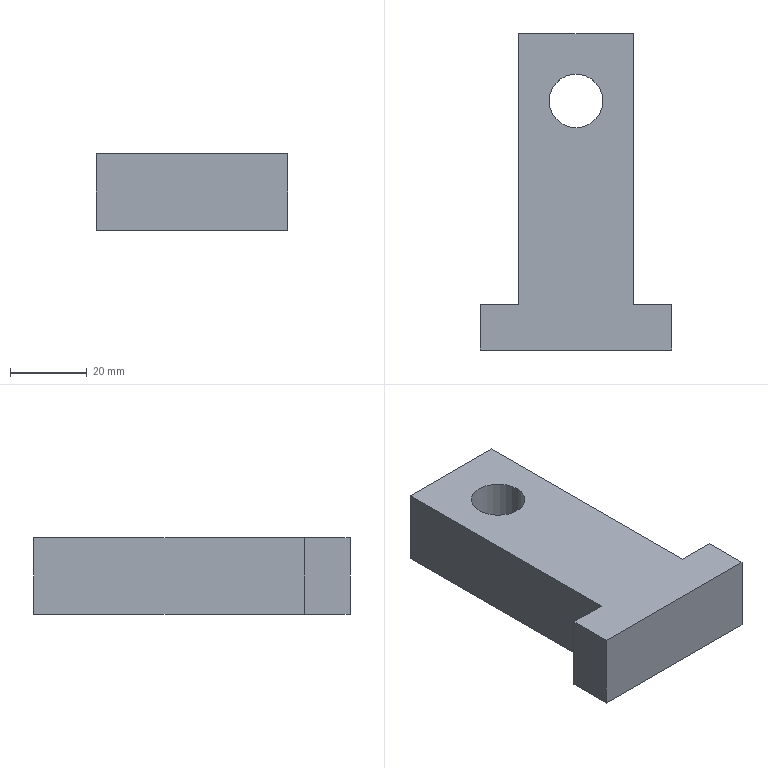Part | SolidWorks | features ICE 2, Extrusion 1 | 1 solid | 12 faces | box 50 x 82.5 x 20 mm | volume 51221 mm3 | plane 10 | cylinder 2 | commonest cylinder face diameters 14 x2
STEP:
#1=CARTESIAN_POINT('',(-7.,23.75,0.));
#2=VERTEX_POINT('',#1);
#3=CARTESIAN_POINT('',(7.,23.75,0.));
#4=VERTEX_POINT('',#3);
#5=CARTESIAN_POINT('',(0.,23.75,0.));
#6=DIRECTION('',(0.,0.,1.));
#7=DIRECTION('',(1.,0.,0.));
#8=AXIS2_PLACEMENT_3D('',#5,#6,#7);
#9=CIRCLE('',#8,7.);
#10=EDGE_CURVE('',#2,#4,#9,.T.);
#11=ORIENTED_EDGE('',*,*,#10,.F.);
#12=CARTESIAN_POINT('',(-7.,23.75,20.));
#13=VERTEX_POINT('',#12);
#14=CARTESIAN_POINT('',(-7.,23.75,0.));
#15=DIRECTION('',(0.,0.,1.));
#16=VECTOR('',#15,1000.);
#17=LINE('',#14,#16);
#18=EDGE_CURVE('',#2,#13,#17,.T.);
#19=ORIENTED_EDGE('',*,*,#18,.T.);
#20=CARTESIAN_POINT('',(7.,23.75,20.));
#21=VERTEX_POINT('',#20);
#22=CARTESIAN_POINT('',(0.,23.75,20.));
#23=DIRECTION('',(0.,0.,1.));
#24=DIRECTION('',(1.,0.,0.));
#25=AXIS2_PLACEMENT_3D('',#22,#23,#24);
#26=CIRCLE('',#25,7.);
#27=EDGE_CURVE('',#13,#21,#26,.T.);
#28=ORIENTED_EDGE('',*,*,#27,.T.);
#29=CARTESIAN_POINT('',(7.,23.75,0.));
#30=DIRECTION('',(0.,0.,1.));
#31=VECTOR('',#30,1000.);
#32=LINE('',#29,#31);
#33=EDGE_CURVE('',#4,#21,#32,.T.);
#34=ORIENTED_EDGE('',*,*,#33,.F.);
#35=EDGE_LOOP('',(#11,#19,#28,#34));
#36=FACE_OUTER_BOUND('',#35,.T.);
#37=CARTESIAN_POINT('',(0.,23.75,0.));
#38=DIRECTION('',(0.,0.,1.));
#39=DIRECTION('',(1.,0.,0.));
#40=AXIS2_PLACEMENT_3D('',#37,#38,#39);
#41=CYLINDRICAL_SURFACE('',#40,7.);
#42=ADVANCED_FACE('',(#36),#41,.F.);
#43=CARTESIAN_POINT('',(25.,-41.25,0.));
#44=VERTEX_POINT('',#43);
#45=CARTESIAN_POINT('',(25.,-29.25,0.));
#46=VERTEX_POINT('',#45);
#47=CARTESIAN_POINT('',(25.,-41.25,0.));
#48=DIRECTION('',(0.,1.,0.));
#49=VECTOR('',#48,1000.);
#50=LINE('',#47,#49);
#51=EDGE_CURVE('',#44,#46,#50,.T.);
#52=ORIENTED_EDGE('',*,*,#51,.T.);
#53=CARTESIAN_POINT('',(25.,-29.25,20.));
#54=VERTEX_POINT('',#53);
#55=CARTESIAN_POINT('',(25.,-29.25,0.));
#56=DIRECTION('',(0.,0.,1.));
#57=VECTOR('',#56,1000.);
#58=LINE('',#55,#57);
#59=EDGE_CURVE('',#46,#54,#58,.T.);
#60=ORIENTED_EDGE('',*,*,#59,.T.);
#61=CARTESIAN_POINT('',(25.,-41.25,20.));
#62=VERTEX_POINT('',#61);
#63=CARTESIAN_POINT('',(25.,-41.25,20.));
#64=DIRECTION('',(0.,1.,0.));
#65=VECTOR('',#64,1000.);
#66=LINE('',#63,#65);
#67=EDGE_CURVE('',#62,#54,#66,.T.);
#68=ORIENTED_EDGE('',*,*,#67,.F.);
#69=CARTESIAN_POINT('',(25.,-41.25,20.));
#70=DIRECTION('',(0.,0.,-1.));
#71=VECTOR('',#70,1000.);
#72=LINE('',#69,#71);
#73=EDGE_CURVE('',#62,#44,#72,.T.);
#74=ORIENTED_EDGE('',*,*,#73,.T.);
#75=EDGE_LOOP('',(#52,#60,#68,#74));
#76=FACE_OUTER_BOUND('',#75,.T.);
#77=CARTESIAN_POINT('',(25.,-41.25,20.));
#78=DIRECTION('',(-1.,0.,0.));
#79=DIRECTION('',(0.,0.,1.));
#80=AXIS2_PLACEMENT_3D('',#77,#78,#79);
#81=PLANE('',#80);
#82=ADVANCED_FACE('',(#76),#81,.F.);
#83=CARTESIAN_POINT('',(15.,41.25,0.));
#84=VERTEX_POINT('',#83);
#85=CARTESIAN_POINT('',(-15.,41.25,0.));
#86=VERTEX_POINT('',#85);
#87=CARTESIAN_POINT('',(-25.,41.25,0.));
#88=DIRECTION('',(-1.,0.,0.));
#89=VECTOR('',#88,1000.);
#90=LINE('',#87,#89);
#91=EDGE_CURVE('',#84,#86,#90,.T.);
#92=ORIENTED_EDGE('',*,*,#91,.T.);
#93=CARTESIAN_POINT('',(-15.,41.25,20.));
#94=VERTEX_POINT('',#93);
#95=CARTESIAN_POINT('',(-15.,41.25,0.));
#96=DIRECTION('',(0.,0.,1.));
#97=VECTOR('',#96,1000.);
#98=LINE('',#95,#97);
#99=EDGE_CURVE('',#86,#94,#98,.T.);
#100=ORIENTED_EDGE('',*,*,#99,.T.);
#101=CARTESIAN_POINT('',(15.,41.25,20.));
#102=VERTEX_POINT('',#101);
#103=CARTESIAN_POINT('',(-25.,41.25,20.));
#104=DIRECTION('',(-1.,0.,0.));
#105=VECTOR('',#104,1000.);
#106=LINE('',#103,#105);
#107=EDGE_CURVE('',#102,#94,#106,.T.);
#108=ORIENTED_EDGE('',*,*,#107,.F.);
#109=CARTESIAN_POINT('',(15.,41.25,0.));
#110=DIRECTION('',(0.,0.,1.));
#111=VECTOR('',#110,1000.);
#112=LINE('',#109,#111);
#113=EDGE_CURVE('',#84,#102,#112,.T.);
#114=ORIENTED_EDGE('',*,*,#113,.F.);
#115=EDGE_LOOP('',(#92,#100,#108,#114));
#116=FACE_OUTER_BOUND('',#115,.T.);
#117=CARTESIAN_POINT('',(-25.,41.25,20.));
#118=DIRECTION('',(0.,-1.,0.));
#119=DIRECTION('',(0.,0.,-1.));
#120=AXIS2_PLACEMENT_3D('',#117,#118,#119);
#121=PLANE('',#120);
#122=ADVANCED_FACE('',(#116),#121,.F.);
#123=CARTESIAN_POINT('',(-25.,-29.25,20.));
#124=VERTEX_POINT('',#123);
#125=CARTESIAN_POINT('',(-25.,-41.25,20.));
#126=VERTEX_POINT('',#125);
#127=CARTESIAN_POINT('',(-25.,-41.25,20.));
#128=DIRECTION('',(0.,-1.,0.));
#129=VECTOR('',#128,1000.);
#130=LINE('',#127,#129);
#131=EDGE_CURVE('',#124,#126,#130,.T.);
#132=ORIENTED_EDGE('',*,*,#131,.F.);
#133=CARTESIAN_POINT('',(-25.,-29.25,0.));
#134=VERTEX_POINT('',#133);
#135=CARTESIAN_POINT('',(-25.,-29.25,0.));
#136=DIRECTION('',(0.,0.,1.));
#137=VECTOR('',#136,1000.);
#138=LINE('',#135,#137);
#139=EDGE_CURVE('',#134,#124,#138,.T.);
#140=ORIENTED_EDGE('',*,*,#139,.F.);
#141=CARTESIAN_POINT('',(-25.,-41.25,0.));
#142=VERTEX_POINT('',#141);
#143=CARTESIAN_POINT('',(-25.,-41.25,0.));
#144=DIRECTION('',(0.,-1.,0.));
#145=VECTOR('',#144,1000.);
#146=LINE('',#143,#145);
#147=EDGE_CURVE('',#134,#142,#146,.T.);
#148=ORIENTED_EDGE('',*,*,#147,.T.);
#149=CARTESIAN_POINT('',(-25.,-41.25,20.));
#150=DIRECTION('',(0.,0.,-1.));
#151=VECTOR('',#150,1000.);
#152=LINE('',#149,#151);
#153=EDGE_CURVE('',#126,#142,#152,.T.);
#154=ORIENTED_EDGE('',*,*,#153,.F.);
#155=EDGE_LOOP('',(#132,#140,#148,#154));
#156=FACE_OUTER_BOUND('',#155,.T.);
#157=CARTESIAN_POINT('',(-25.,-41.25,20.));
#158=DIRECTION('',(1.,0.,0.));
#159=DIRECTION('',(0.,0.,-1.));
#160=AXIS2_PLACEMENT_3D('',#157,#158,#159);
#161=PLANE('',#160);
#162=ADVANCED_FACE('',(#156),#161,.F.);
#163=CARTESIAN_POINT('',(-25.,-41.25,0.));
#164=DIRECTION('',(1.,0.,0.));
#165=VECTOR('',#164,1000.);
#166=LINE('',#163,#165);
#167=EDGE_CURVE('',#142,#44,#166,.T.);
#168=ORIENTED_EDGE('',*,*,#167,.T.);
#169=ORIENTED_EDGE('',*,*,#73,.F.);
#170=CARTESIAN_POINT('',(-25.,-41.25,20.));
#171=DIRECTION('',(1.,0.,0.));
#172=VECTOR('',#171,1000.);
#173=LINE('',#170,#172);
#174=EDGE_CURVE('',#126,#62,#173,.T.);
#175=ORIENTED_EDGE('',*,*,#174,.F.);
#176=ORIENTED_EDGE('',*,*,#153,.T.);
#177=EDGE_LOOP('',(#168,#169,#175,#176));
#178=FACE_OUTER_BOUND('',#177,.T.);
#179=CARTESIAN_POINT('',(-25.,-41.25,20.));
#180=DIRECTION('',(0.,1.,0.));
#181=DIRECTION('',(0.,0.,1.));
#182=AXIS2_PLACEMENT_3D('',#179,#180,#181);
#183=PLANE('',#182);
#184=ADVANCED_FACE('',(#178),#183,.F.);
#185=CARTESIAN_POINT('',(0.,23.75,20.));
#186=DIRECTION('',(0.,0.,1.));
#187=DIRECTION('',(1.,0.,0.));
#188=AXIS2_PLACEMENT_3D('',#185,#186,#187);
#189=CIRCLE('',#188,7.);
#190=EDGE_CURVE('',#21,#13,#189,.T.);
#191=ORIENTED_EDGE('',*,*,#190,.F.);
#192=ORIENTED_EDGE('',*,*,#27,.F.);
#193=EDGE_LOOP('',(#191,#192));
#194=FACE_BOUND('',#193,.T.);
#195=ORIENTED_EDGE('',*,*,#107,.T.);
#196=CARTESIAN_POINT('',(-15.,-29.25,20.));
#197=VERTEX_POINT('',#196);
#198=CARTESIAN_POINT('',(-15.,41.25,20.));
#199=DIRECTION('',(0.,1.,0.));
#200=VECTOR('',#199,1000.);
#201=LINE('',#198,#200);
#202=EDGE_CURVE('',#197,#94,#201,.T.);
#203=ORIENTED_EDGE('',*,*,#202,.F.);
#204=CARTESIAN_POINT('',(-25.,-29.25,20.));
#205=DIRECTION('',(1.,0.,0.));
#206=VECTOR('',#205,1000.);
#207=LINE('',#204,#206);
#208=EDGE_CURVE('',#124,#197,#207,.T.);
#209=ORIENTED_EDGE('',*,*,#208,.F.);
#210=ORIENTED_EDGE('',*,*,#131,.T.);
#211=ORIENTED_EDGE('',*,*,#174,.T.);
#212=ORIENTED_EDGE('',*,*,#67,.T.);
#213=CARTESIAN_POINT('',(15.,-29.25,20.));
#214=VERTEX_POINT('',#213);
#215=CARTESIAN_POINT('',(25.,-29.25,20.));
#216=DIRECTION('',(1.,0.,0.));
#217=VECTOR('',#216,1000.);
#218=LINE('',#215,#217);
#219=EDGE_CURVE('',#214,#54,#218,.T.);
#220=ORIENTED_EDGE('',*,*,#219,.F.);
#221=CARTESIAN_POINT('',(15.,41.25,20.));
#222=DIRECTION('',(0.,-1.,0.));
#223=VECTOR('',#222,1000.);
#224=LINE('',#221,#223);
#225=EDGE_CURVE('',#102,#214,#224,.T.);
#226=ORIENTED_EDGE('',*,*,#225,.F.);
#227=EDGE_LOOP('',(#195,#203,#209,#210,#211,#212,#220,#226));
#228=FACE_OUTER_BOUND('',#227,.T.);
#229=CARTESIAN_POINT('',(0.,0.,20.));
#230=DIRECTION('',(0.,0.,-1.));
#231=DIRECTION('',(-1.,0.,0.));
#232=AXIS2_PLACEMENT_3D('',#229,#230,#231);
#233=PLANE('',#232);
#234=ADVANCED_FACE('',(#194,#228),#233,.F.);
#235=CARTESIAN_POINT('',(-15.,-29.25,0.));
#236=VERTEX_POINT('',#235);
#237=CARTESIAN_POINT('',(-15.,41.25,0.));
#238=DIRECTION('',(0.,1.,0.));
#239=VECTOR('',#238,1000.);
#240=LINE('',#237,#239);
#241=EDGE_CURVE('',#236,#86,#240,.T.);
#242=ORIENTED_EDGE('',*,*,#241,.T.);
#243=ORIENTED_EDGE('',*,*,#91,.F.);
#244=CARTESIAN_POINT('',(15.,-29.25,0.));
#245=VERTEX_POINT('',#244);
#246=CARTESIAN_POINT('',(15.,41.25,0.));
#247=DIRECTION('',(0.,-1.,0.));
#248=VECTOR('',#247,1000.);
#249=LINE('',#246,#248);
#250=EDGE_CURVE('',#84,#245,#249,.T.);
#251=ORIENTED_EDGE('',*,*,#250,.T.);
#252=CARTESIAN_POINT('',(25.,-29.25,0.));
#253=DIRECTION('',(1.,0.,0.));
#254=VECTOR('',#253,1000.);
#255=LINE('',#252,#254);
#256=EDGE_CURVE('',#245,#46,#255,.T.);
#257=ORIENTED_EDGE('',*,*,#256,.T.);
#258=ORIENTED_EDGE('',*,*,#51,.F.);
#259=ORIENTED_EDGE('',*,*,#167,.F.);
#260=ORIENTED_EDGE('',*,*,#147,.F.);
#261=CARTESIAN_POINT('',(-25.,-29.25,0.));
#262=DIRECTION('',(1.,0.,0.));
#263=VECTOR('',#262,1000.);
#264=LINE('',#261,#263);
#265=EDGE_CURVE('',#134,#236,#264,.T.);
#266=ORIENTED_EDGE('',*,*,#265,.T.);
#267=EDGE_LOOP('',(#242,#243,#251,#257,#258,#259,#260,#266));
#268=FACE_OUTER_BOUND('',#267,.T.);
#269=CARTESIAN_POINT('',(0.,23.75,0.));
#270=DIRECTION('',(0.,0.,1.));
#271=DIRECTION('',(1.,0.,0.));
#272=AXIS2_PLACEMENT_3D('',#269,#270,#271);
#273=CIRCLE('',#272,7.);
#274=EDGE_CURVE('',#4,#2,#273,.T.);
#275=ORIENTED_EDGE('',*,*,#274,.T.);
#276=ORIENTED_EDGE('',*,*,#10,.T.);
#277=EDGE_LOOP('',(#275,#276));
#278=FACE_BOUND('',#277,.T.);
#279=CARTESIAN_POINT('',(0.,0.,0.));
#280=DIRECTION('',(0.,0.,-1.));
#281=DIRECTION('',(-1.,0.,0.));
#282=AXIS2_PLACEMENT_3D('',#279,#280,#281);
#283=PLANE('',#282);
#284=ADVANCED_FACE('',(#268,#278),#283,.T.);
#285=ORIENTED_EDGE('',*,*,#18,.F.);
#286=ORIENTED_EDGE('',*,*,#274,.F.);
#287=ORIENTED_EDGE('',*,*,#33,.T.);
#288=ORIENTED_EDGE('',*,*,#190,.T.);
#289=EDGE_LOOP('',(#285,#286,#287,#288));
#290=FACE_OUTER_BOUND('',#289,.T.);
#291=CARTESIAN_POINT('',(0.,23.75,0.));
#292=DIRECTION('',(0.,0.,1.));
#293=DIRECTION('',(1.,0.,0.));
#294=AXIS2_PLACEMENT_3D('',#291,#292,#293);
#295=CYLINDRICAL_SURFACE('',#294,7.);
#296=ADVANCED_FACE('',(#290),#295,.F.);
#297=ORIENTED_EDGE('',*,*,#219,.T.);
#298=ORIENTED_EDGE('',*,*,#59,.F.);
#299=ORIENTED_EDGE('',*,*,#256,.F.);
#300=CARTESIAN_POINT('',(15.,-29.25,0.));
#301=DIRECTION('',(0.,0.,1.));
#302=VECTOR('',#301,1000.);
#303=LINE('',#300,#302);
#304=EDGE_CURVE('',#245,#214,#303,.T.);
#305=ORIENTED_EDGE('',*,*,#304,.T.);
#306=EDGE_LOOP('',(#297,#298,#299,#305));
#307=FACE_OUTER_BOUND('',#306,.T.);
#308=CARTESIAN_POINT('',(25.,-29.25,0.));
#309=DIRECTION('',(0.,-1.,0.));
#310=DIRECTION('',(1.,0.,0.));
#311=AXIS2_PLACEMENT_3D('',#308,#309,#310);
#312=PLANE('',#311);
#313=ADVANCED_FACE('',(#307),#312,.F.);
#314=ORIENTED_EDGE('',*,*,#225,.T.);
#315=ORIENTED_EDGE('',*,*,#304,.F.);
#316=ORIENTED_EDGE('',*,*,#250,.F.);
#317=ORIENTED_EDGE('',*,*,#113,.T.);
#318=EDGE_LOOP('',(#314,#315,#316,#317));
#319=FACE_OUTER_BOUND('',#318,.T.);
#320=CARTESIAN_POINT('',(15.,41.25,0.));
#321=DIRECTION('',(-1.,0.,0.));
#322=DIRECTION('',(0.,-1.,0.));
#323=AXIS2_PLACEMENT_3D('',#320,#321,#322);
#324=PLANE('',#323);
#325=ADVANCED_FACE('',(#319),#324,.F.);
#326=ORIENTED_EDGE('',*,*,#202,.T.);
#327=ORIENTED_EDGE('',*,*,#99,.F.);
#328=ORIENTED_EDGE('',*,*,#241,.F.);
#329=CARTESIAN_POINT('',(-15.,-29.25,0.));
#330=DIRECTION('',(0.,0.,1.));
#331=VECTOR('',#330,1000.);
#332=LINE('',#329,#331);
#333=EDGE_CURVE('',#236,#197,#332,.T.);
#334=ORIENTED_EDGE('',*,*,#333,.T.);
#335=EDGE_LOOP('',(#326,#327,#328,#334));
#336=FACE_OUTER_BOUND('',#335,.T.);
#337=CARTESIAN_POINT('',(-15.,41.25,0.));
#338=DIRECTION('',(1.,0.,0.));
#339=DIRECTION('',(0.,1.,0.));
#340=AXIS2_PLACEMENT_3D('',#337,#338,#339);
#341=PLANE('',#340);
#342=ADVANCED_FACE('',(#336),#341,.F.);
#343=ORIENTED_EDGE('',*,*,#208,.T.);
#344=ORIENTED_EDGE('',*,*,#333,.F.);
#345=ORIENTED_EDGE('',*,*,#265,.F.);
#346=ORIENTED_EDGE('',*,*,#139,.T.);
#347=EDGE_LOOP('',(#343,#344,#345,#346));
#348=FACE_OUTER_BOUND('',#347,.T.);
#349=CARTESIAN_POINT('',(-25.,-29.25,0.));
#350=DIRECTION('',(0.,-1.,0.));
#351=DIRECTION('',(1.,0.,0.));
#352=AXIS2_PLACEMENT_3D('',#349,#350,#351);
#353=PLANE('',#352);
#354=ADVANCED_FACE('',(#348),#353,.F.);
#355=CLOSED_SHELL('',(#42,#82,#122,#162,#184,#234,#284,#296,#313,#325,#342,#354));
#356=MANIFOLD_SOLID_BREP('',#355);
#357=CARTESIAN_POINT('',(0.,0.,0.));
#358=DIRECTION('',(0.,0.,1.));
#359=DIRECTION('',(1.,0.,0.));
#360=AXIS2_PLACEMENT_3D('',#357,#358,#359);
#361=(LENGTH_UNIT()NAMED_UNIT(*)SI_UNIT(.MILLI.,.METRE.));
#362=UNCERTAINTY_MEASURE_WITH_UNIT(LENGTH_MEASURE(0.00001),#361,'','');
#363=(NAMED_UNIT(*)PLANE_ANGLE_UNIT()SI_UNIT($,.RADIAN.));
#364=(NAMED_UNIT(*)SI_UNIT($,.STERADIAN.)SOLID_ANGLE_UNIT());
#365=(GEOMETRIC_REPRESENTATION_CONTEXT(3)GLOBAL_UNCERTAINTY_ASSIGNED_CONTEXT((#362))GLOBAL_UNIT_ASSIGNED_CONTEXT((#361,#363,#364))REPRESENTATION_CONTEXT('',''));
#366=ADVANCED_BREP_SHAPE_REPRESENTATION('',(#356,#360),#365);